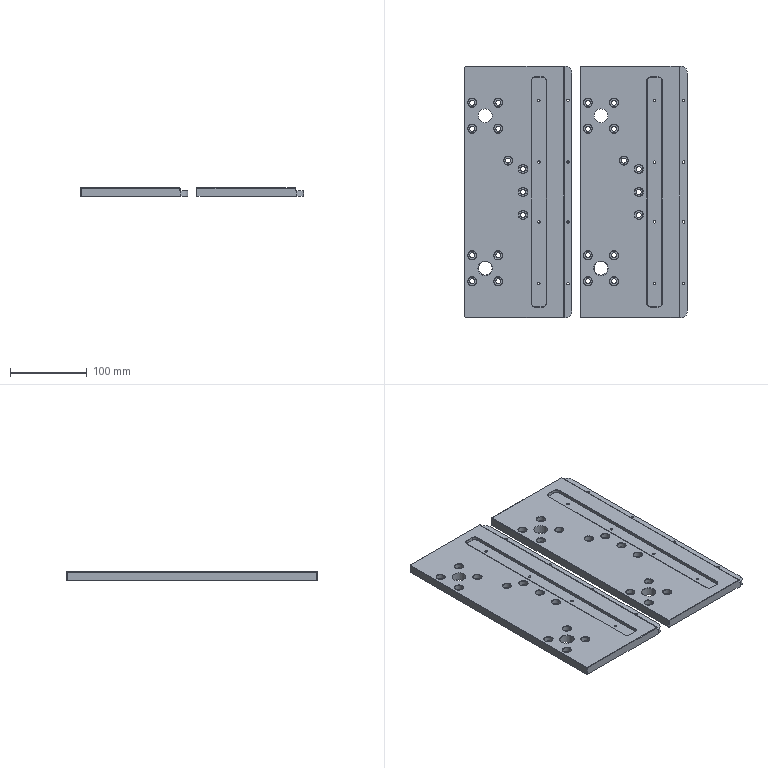Part | 2 solids | 196 faces | box 291 x 328 x 11 mm | volume 904466 mm3 | cylinder 82 | plane 76 | cone 38 | commonest cylinder face diameters 6.5 x24 11 x24 3.2 x16 10.1 x8 18 x8 2 x2